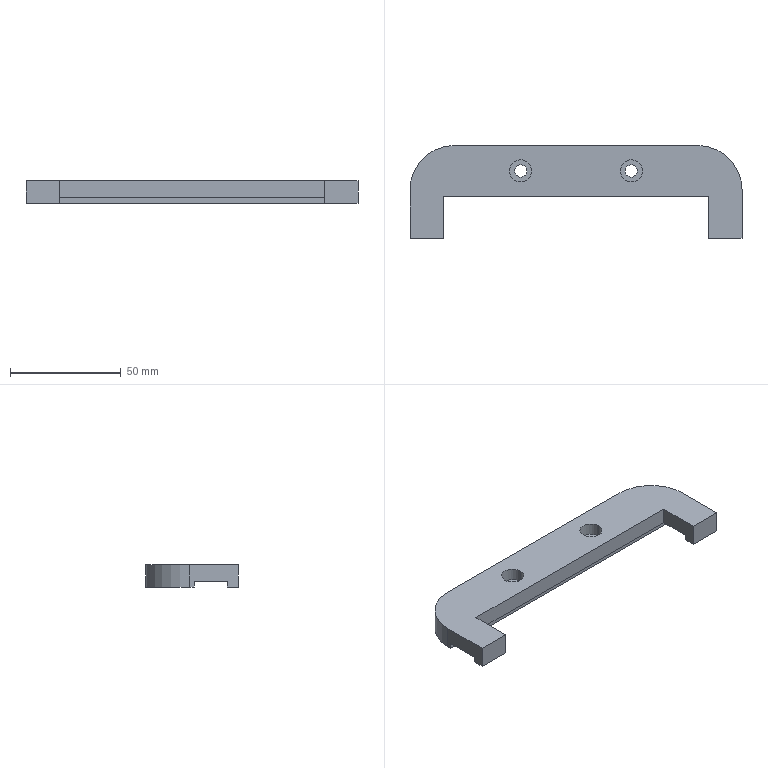Part | STEP file | X77-04403 | 1 solid | 28 faces | box 150 x 42 x 10 mm | volume 35959 mm3 | plane 18 | cylinder 10 | commonest cylinder face diameters 5.5 x4 10 x4 40 x2
STEP:
#1=CARTESIAN_POINT('',(45.,30.5,4.3));
#2=VERTEX_POINT('',#1);
#3=CARTESIAN_POINT('',(55.,30.5,4.3));
#4=VERTEX_POINT('',#3);
#5=CARTESIAN_POINT('',(50.,30.5,4.3));
#6=DIRECTION('',(0.,0.,1.));
#7=DIRECTION('',(1.,0.,0.));
#8=AXIS2_PLACEMENT_3D('',#5,#6,#7);
#9=CIRCLE('',#8,5.);
#10=EDGE_CURVE('',#2,#4,#9,.T.);
#11=ORIENTED_EDGE('',*,*,#10,.F.);
#12=CARTESIAN_POINT('',(45.,30.5,10.));
#13=VERTEX_POINT('',#12);
#14=CARTESIAN_POINT('',(45.,30.5,10.));
#15=DIRECTION('',(0.,0.,1.));
#16=VECTOR('',#15,1000.);
#17=LINE('',#14,#16);
#18=EDGE_CURVE('',#2,#13,#17,.T.);
#19=ORIENTED_EDGE('',*,*,#18,.T.);
#20=CARTESIAN_POINT('',(55.,30.5,10.));
#21=VERTEX_POINT('',#20);
#22=CARTESIAN_POINT('',(50.,30.5,10.));
#23=DIRECTION('',(0.,0.,1.));
#24=DIRECTION('',(1.,0.,0.));
#25=AXIS2_PLACEMENT_3D('',#22,#23,#24);
#26=CIRCLE('',#25,5.);
#27=EDGE_CURVE('',#13,#21,#26,.T.);
#28=ORIENTED_EDGE('',*,*,#27,.T.);
#29=CARTESIAN_POINT('',(55.,30.5,10.));
#30=DIRECTION('',(0.,0.,1.));
#31=VECTOR('',#30,1000.);
#32=LINE('',#29,#31);
#33=EDGE_CURVE('',#4,#21,#32,.T.);
#34=ORIENTED_EDGE('',*,*,#33,.F.);
#35=EDGE_LOOP('',(#11,#19,#28,#34));
#36=FACE_OUTER_BOUND('',#35,.T.);
#37=CARTESIAN_POINT('',(50.,30.5,10.));
#38=DIRECTION('',(0.,0.,1.));
#39=DIRECTION('',(1.,0.,0.));
#40=AXIS2_PLACEMENT_3D('',#37,#38,#39);
#41=CYLINDRICAL_SURFACE('',#40,5.);
#42=ADVANCED_FACE('',(#36),#41,.F.);
#43=CARTESIAN_POINT('',(47.25,30.5,0.));
#44=VERTEX_POINT('',#43);
#45=CARTESIAN_POINT('',(52.75,30.5,0.));
#46=VERTEX_POINT('',#45);
#47=CARTESIAN_POINT('',(50.,30.5,0.));
#48=DIRECTION('',(0.,0.,1.));
#49=DIRECTION('',(1.,0.,0.));
#50=AXIS2_PLACEMENT_3D('',#47,#48,#49);
#51=CIRCLE('',#50,2.75);
#52=EDGE_CURVE('',#44,#46,#51,.T.);
#53=ORIENTED_EDGE('',*,*,#52,.F.);
#54=CARTESIAN_POINT('',(47.25,30.5,4.3));
#55=VERTEX_POINT('',#54);
#56=CARTESIAN_POINT('',(47.25,30.5,10.));
#57=DIRECTION('',(0.,0.,1.));
#58=VECTOR('',#57,1000.);
#59=LINE('',#56,#58);
#60=EDGE_CURVE('',#44,#55,#59,.T.);
#61=ORIENTED_EDGE('',*,*,#60,.T.);
#62=CARTESIAN_POINT('',(52.75,30.5,4.3));
#63=VERTEX_POINT('',#62);
#64=CARTESIAN_POINT('',(50.,30.5,4.3));
#65=DIRECTION('',(0.,0.,1.));
#66=DIRECTION('',(1.,0.,0.));
#67=AXIS2_PLACEMENT_3D('',#64,#65,#66);
#68=CIRCLE('',#67,2.75);
#69=EDGE_CURVE('',#55,#63,#68,.T.);
#70=ORIENTED_EDGE('',*,*,#69,.T.);
#71=CARTESIAN_POINT('',(52.75,30.5,10.));
#72=DIRECTION('',(0.,0.,1.));
#73=VECTOR('',#72,1000.);
#74=LINE('',#71,#73);
#75=EDGE_CURVE('',#46,#63,#74,.T.);
#76=ORIENTED_EDGE('',*,*,#75,.F.);
#77=EDGE_LOOP('',(#53,#61,#70,#76));
#78=FACE_OUTER_BOUND('',#77,.T.);
#79=CARTESIAN_POINT('',(50.,30.5,10.));
#80=DIRECTION('',(0.,0.,1.));
#81=DIRECTION('',(1.,0.,0.));
#82=AXIS2_PLACEMENT_3D('',#79,#80,#81);
#83=CYLINDRICAL_SURFACE('',#82,2.75);
#84=ADVANCED_FACE('',(#78),#83,.F.);
#85=CARTESIAN_POINT('',(95.,30.5,4.3));
#86=VERTEX_POINT('',#85);
#87=CARTESIAN_POINT('',(105.,30.5,4.3));
#88=VERTEX_POINT('',#87);
#89=CARTESIAN_POINT('',(100.,30.5,4.3));
#90=DIRECTION('',(0.,0.,1.));
#91=DIRECTION('',(1.,0.,0.));
#92=AXIS2_PLACEMENT_3D('',#89,#90,#91);
#93=CIRCLE('',#92,5.);
#94=EDGE_CURVE('',#86,#88,#93,.T.);
#95=ORIENTED_EDGE('',*,*,#94,.F.);
#96=CARTESIAN_POINT('',(95.,30.5,10.));
#97=VERTEX_POINT('',#96);
#98=CARTESIAN_POINT('',(95.,30.5,10.));
#99=DIRECTION('',(0.,0.,1.));
#100=VECTOR('',#99,1000.);
#101=LINE('',#98,#100);
#102=EDGE_CURVE('',#86,#97,#101,.T.);
#103=ORIENTED_EDGE('',*,*,#102,.T.);
#104=CARTESIAN_POINT('',(105.,30.5,10.));
#105=VERTEX_POINT('',#104);
#106=CARTESIAN_POINT('',(100.,30.5,10.));
#107=DIRECTION('',(0.,0.,1.));
#108=DIRECTION('',(1.,0.,0.));
#109=AXIS2_PLACEMENT_3D('',#106,#107,#108);
#110=CIRCLE('',#109,5.);
#111=EDGE_CURVE('',#97,#105,#110,.T.);
#112=ORIENTED_EDGE('',*,*,#111,.T.);
#113=CARTESIAN_POINT('',(105.,30.5,10.));
#114=DIRECTION('',(0.,0.,1.));
#115=VECTOR('',#114,1000.);
#116=LINE('',#113,#115);
#117=EDGE_CURVE('',#88,#105,#116,.T.);
#118=ORIENTED_EDGE('',*,*,#117,.F.);
#119=EDGE_LOOP('',(#95,#103,#112,#118));
#120=FACE_OUTER_BOUND('',#119,.T.);
#121=CARTESIAN_POINT('',(100.,30.5,10.));
#122=DIRECTION('',(0.,0.,1.));
#123=DIRECTION('',(1.,0.,0.));
#124=AXIS2_PLACEMENT_3D('',#121,#122,#123);
#125=CYLINDRICAL_SURFACE('',#124,5.);
#126=ADVANCED_FACE('',(#120),#125,.F.);
#127=CARTESIAN_POINT('',(97.25,30.5,0.));
#128=VERTEX_POINT('',#127);
#129=CARTESIAN_POINT('',(102.75,30.5,0.));
#130=VERTEX_POINT('',#129);
#131=CARTESIAN_POINT('',(100.,30.5,0.));
#132=DIRECTION('',(0.,0.,1.));
#133=DIRECTION('',(1.,0.,0.));
#134=AXIS2_PLACEMENT_3D('',#131,#132,#133);
#135=CIRCLE('',#134,2.75);
#136=EDGE_CURVE('',#128,#130,#135,.T.);
#137=ORIENTED_EDGE('',*,*,#136,.F.);
#138=CARTESIAN_POINT('',(97.25,30.5,4.3));
#139=VERTEX_POINT('',#138);
#140=CARTESIAN_POINT('',(97.25,30.5,10.));
#141=DIRECTION('',(0.,0.,1.));
#142=VECTOR('',#141,1000.);
#143=LINE('',#140,#142);
#144=EDGE_CURVE('',#128,#139,#143,.T.);
#145=ORIENTED_EDGE('',*,*,#144,.T.);
#146=CARTESIAN_POINT('',(102.75,30.5,4.3));
#147=VERTEX_POINT('',#146);
#148=CARTESIAN_POINT('',(100.,30.5,4.3));
#149=DIRECTION('',(0.,0.,1.));
#150=DIRECTION('',(1.,0.,0.));
#151=AXIS2_PLACEMENT_3D('',#148,#149,#150);
#152=CIRCLE('',#151,2.75);
#153=EDGE_CURVE('',#139,#147,#152,.T.);
#154=ORIENTED_EDGE('',*,*,#153,.T.);
#155=CARTESIAN_POINT('',(102.75,30.5,10.));
#156=DIRECTION('',(0.,0.,1.));
#157=VECTOR('',#156,1000.);
#158=LINE('',#155,#157);
#159=EDGE_CURVE('',#130,#147,#158,.T.);
#160=ORIENTED_EDGE('',*,*,#159,.F.);
#161=EDGE_LOOP('',(#137,#145,#154,#160));
#162=FACE_OUTER_BOUND('',#161,.T.);
#163=CARTESIAN_POINT('',(100.,30.5,10.));
#164=DIRECTION('',(0.,0.,1.));
#165=DIRECTION('',(1.,0.,0.));
#166=AXIS2_PLACEMENT_3D('',#163,#164,#165);
#167=CYLINDRICAL_SURFACE('',#166,2.75);
#168=ADVANCED_FACE('',(#162),#167,.F.);
#169=CARTESIAN_POINT('',(150.,5.,0.));
#170=VERTEX_POINT('',#169);
#171=CARTESIAN_POINT('',(135.,5.,0.));
#172=VERTEX_POINT('',#171);
#173=CARTESIAN_POINT('',(0.,5.,0.));
#174=DIRECTION('',(-1.,0.,0.));
#175=VECTOR('',#174,1000.);
#176=LINE('',#173,#175);
#177=EDGE_CURVE('',#170,#172,#176,.T.);
#178=ORIENTED_EDGE('',*,*,#177,.F.);
#179=CARTESIAN_POINT('',(150.,0.,0.));
#180=VERTEX_POINT('',#179);
#181=CARTESIAN_POINT('',(150.,0.,0.));
#182=DIRECTION('',(0.,1.,0.));
#183=VECTOR('',#182,1000.);
#184=LINE('',#181,#183);
#185=EDGE_CURVE('',#180,#170,#184,.T.);
#186=ORIENTED_EDGE('',*,*,#185,.F.);
#187=CARTESIAN_POINT('',(135.,0.,0.));
#188=VERTEX_POINT('',#187);
#189=CARTESIAN_POINT('',(135.,0.,0.));
#190=DIRECTION('',(1.,0.,0.));
#191=VECTOR('',#190,1000.);
#192=LINE('',#189,#191);
#193=EDGE_CURVE('',#188,#180,#192,.T.);
#194=ORIENTED_EDGE('',*,*,#193,.F.);
#195=CARTESIAN_POINT('',(135.,0.,0.));
#196=DIRECTION('',(0.,-1.,0.));
#197=VECTOR('',#196,1000.);
#198=LINE('',#195,#197);
#199=EDGE_CURVE('',#172,#188,#198,.T.);
#200=ORIENTED_EDGE('',*,*,#199,.F.);
#201=EDGE_LOOP('',(#178,#186,#194,#200));
#202=FACE_OUTER_BOUND('',#201,.T.);
#203=CARTESIAN_POINT('',(0.,42.,0.));
#204=DIRECTION('',(0.,0.,-1.));
#205=DIRECTION('',(-1.,0.,0.));
#206=AXIS2_PLACEMENT_3D('',#203,#204,#205);
#207=PLANE('',#206);
#208=ADVANCED_FACE('',(#202),#207,.T.);
#209=CARTESIAN_POINT('',(15.,5.,0.));
#210=VERTEX_POINT('',#209);
#211=CARTESIAN_POINT('',(0.,5.,0.));
#212=VERTEX_POINT('',#211);
#213=CARTESIAN_POINT('',(0.,5.,0.));
#214=DIRECTION('',(-1.,0.,0.));
#215=VECTOR('',#214,1000.);
#216=LINE('',#213,#215);
#217=EDGE_CURVE('',#210,#212,#216,.T.);
#218=ORIENTED_EDGE('',*,*,#217,.F.);
#219=CARTESIAN_POINT('',(15.,0.,0.));
#220=VERTEX_POINT('',#219);
#221=CARTESIAN_POINT('',(15.,0.,0.));
#222=DIRECTION('',(0.,1.,0.));
#223=VECTOR('',#222,1000.);
#224=LINE('',#221,#223);
#225=EDGE_CURVE('',#220,#210,#224,.T.);
#226=ORIENTED_EDGE('',*,*,#225,.F.);
#227=CARTESIAN_POINT('',(0.,0.,0.));
#228=VERTEX_POINT('',#227);
#229=CARTESIAN_POINT('',(0.,0.,0.));
#230=DIRECTION('',(1.,0.,0.));
#231=VECTOR('',#230,1000.);
#232=LINE('',#229,#231);
#233=EDGE_CURVE('',#228,#220,#232,.T.);
#234=ORIENTED_EDGE('',*,*,#233,.F.);
#235=CARTESIAN_POINT('',(0.,0.,0.));
#236=DIRECTION('',(0.,-1.,0.));
#237=VECTOR('',#236,1000.);
#238=LINE('',#235,#237);
#239=EDGE_CURVE('',#212,#228,#238,.T.);
#240=ORIENTED_EDGE('',*,*,#239,.F.);
#241=EDGE_LOOP('',(#218,#226,#234,#240));
#242=FACE_OUTER_BOUND('',#241,.T.);
#243=CARTESIAN_POINT('',(0.,42.,0.));
#244=DIRECTION('',(0.,0.,-1.));
#245=DIRECTION('',(-1.,0.,0.));
#246=AXIS2_PLACEMENT_3D('',#243,#244,#245);
#247=PLANE('',#246);
#248=ADVANCED_FACE('',(#242),#247,.T.);
#249=CARTESIAN_POINT('',(0.,22.,10.));
#250=VERTEX_POINT('',#249);
#251=CARTESIAN_POINT('',(0.,0.,10.));
#252=VERTEX_POINT('',#251);
#253=CARTESIAN_POINT('',(0.,0.,10.));
#254=DIRECTION('',(0.,-1.,0.));
#255=VECTOR('',#254,1000.);
#256=LINE('',#253,#255);
#257=EDGE_CURVE('',#250,#252,#256,.T.);
#258=ORIENTED_EDGE('',*,*,#257,.F.);
#259=CARTESIAN_POINT('',(0.,22.,0.));
#260=VERTEX_POINT('',#259);
#261=CARTESIAN_POINT('',(0.,22.,10.));
#262=DIRECTION('',(0.,0.,-1.));
#263=VECTOR('',#262,1000.);
#264=LINE('',#261,#263);
#265=EDGE_CURVE('',#250,#260,#264,.T.);
#266=ORIENTED_EDGE('',*,*,#265,.T.);
#267=CARTESIAN_POINT('',(0.,20.,0.));
#268=VERTEX_POINT('',#267);
#269=CARTESIAN_POINT('',(0.,0.,0.));
#270=DIRECTION('',(0.,-1.,0.));
#271=VECTOR('',#270,1000.);
#272=LINE('',#269,#271);
#273=EDGE_CURVE('',#260,#268,#272,.T.);
#274=ORIENTED_EDGE('',*,*,#273,.T.);
#275=CARTESIAN_POINT('',(0.,20.,2.5));
#276=VERTEX_POINT('',#275);
#277=CARTESIAN_POINT('',(0.,20.,10.));
#278=DIRECTION('',(0.,0.,1.));
#279=VECTOR('',#278,1000.);
#280=LINE('',#277,#279);
#281=EDGE_CURVE('',#268,#276,#280,.T.);
#282=ORIENTED_EDGE('',*,*,#281,.T.);
#283=CARTESIAN_POINT('',(0.,5.,2.5));
#284=VERTEX_POINT('',#283);
#285=CARTESIAN_POINT('',(0.,0.,2.5));
#286=DIRECTION('',(0.,-1.,0.));
#287=VECTOR('',#286,1000.);
#288=LINE('',#285,#287);
#289=EDGE_CURVE('',#276,#284,#288,.T.);
#290=ORIENTED_EDGE('',*,*,#289,.T.);
#291=CARTESIAN_POINT('',(0.,5.,10.));
#292=DIRECTION('',(0.,0.,-1.));
#293=VECTOR('',#292,1000.);
#294=LINE('',#291,#293);
#295=EDGE_CURVE('',#284,#212,#294,.T.);
#296=ORIENTED_EDGE('',*,*,#295,.T.);
#297=ORIENTED_EDGE('',*,*,#239,.T.);
#298=CARTESIAN_POINT('',(0.,0.,10.));
#299=DIRECTION('',(0.,0.,-1.));
#300=VECTOR('',#299,1000.);
#301=LINE('',#298,#300);
#302=EDGE_CURVE('',#252,#228,#301,.T.);
#303=ORIENTED_EDGE('',*,*,#302,.F.);
#304=EDGE_LOOP('',(#258,#266,#274,#282,#290,#296,#297,#303));
#305=FACE_OUTER_BOUND('',#304,.T.);
#306=CARTESIAN_POINT('',(0.,0.,10.));
#307=DIRECTION('',(1.,0.,0.));
#308=DIRECTION('',(0.,0.,-1.));
#309=AXIS2_PLACEMENT_3D('',#306,#307,#308);
#310=PLANE('',#309);
#311=ADVANCED_FACE('',(#305),#310,.F.);
#312=ORIENTED_EDGE('',*,*,#233,.T.);
#313=CARTESIAN_POINT('',(15.,0.,10.));
#314=VERTEX_POINT('',#313);
#315=CARTESIAN_POINT('',(15.,0.,10.));
#316=DIRECTION('',(0.,0.,-1.));
#317=VECTOR('',#316,1000.);
#318=LINE('',#315,#317);
#319=EDGE_CURVE('',#314,#220,#318,.T.);
#320=ORIENTED_EDGE('',*,*,#319,.F.);
#321=CARTESIAN_POINT('',(0.,0.,10.));
#322=DIRECTION('',(1.,0.,0.));
#323=VECTOR('',#322,1000.);
#324=LINE('',#321,#323);
#325=EDGE_CURVE('',#252,#314,#324,.T.);
#326=ORIENTED_EDGE('',*,*,#325,.F.);
#327=ORIENTED_EDGE('',*,*,#302,.T.);
#328=EDGE_LOOP('',(#312,#320,#326,#327));
#329=FACE_OUTER_BOUND('',#328,.T.);
#330=CARTESIAN_POINT('',(0.,0.,10.));
#331=DIRECTION('',(0.,1.,0.));
#332=DIRECTION('',(0.,0.,1.));
#333=AXIS2_PLACEMENT_3D('',#330,#331,#332);
#334=PLANE('',#333);
#335=ADVANCED_FACE('',(#329),#334,.F.);
#336=ORIENTED_EDGE('',*,*,#225,.T.);
#337=CARTESIAN_POINT('',(15.,5.,2.5));
#338=VERTEX_POINT('',#337);
#339=CARTESIAN_POINT('',(15.,5.,10.));
#340=DIRECTION('',(0.,0.,1.));
#341=VECTOR('',#340,1000.);
#342=LINE('',#339,#341);
#343=EDGE_CURVE('',#210,#338,#342,.T.);
#344=ORIENTED_EDGE('',*,*,#343,.T.);
#345=CARTESIAN_POINT('',(15.,19.,2.5));
#346=VERTEX_POINT('',#345);
#347=CARTESIAN_POINT('',(15.,0.,2.5));
#348=DIRECTION('',(0.,1.,0.));
#349=VECTOR('',#348,1000.);
#350=LINE('',#347,#349);
#351=EDGE_CURVE('',#338,#346,#350,.T.);
#352=ORIENTED_EDGE('',*,*,#351,.T.);
#353=CARTESIAN_POINT('',(15.,19.,10.));
#354=VERTEX_POINT('',#353);
#355=CARTESIAN_POINT('',(15.,19.,10.));
#356=DIRECTION('',(0.,0.,-1.));
#357=VECTOR('',#356,1000.);
#358=LINE('',#355,#357);
#359=EDGE_CURVE('',#354,#346,#358,.T.);
#360=ORIENTED_EDGE('',*,*,#359,.F.);
#361=CARTESIAN_POINT('',(15.,0.,10.));
#362=DIRECTION('',(0.,1.,0.));
#363=VECTOR('',#362,1000.);
#364=LINE('',#361,#363);
#365=EDGE_CURVE('',#314,#354,#364,.T.);
#366=ORIENTED_EDGE('',*,*,#365,.F.);
#367=ORIENTED_EDGE('',*,*,#319,.T.);
#368=EDGE_LOOP('',(#336,#344,#352,#360,#366,#367));
#369=FACE_OUTER_BOUND('',#368,.T.);
#370=CARTESIAN_POINT('',(15.,0.,10.));
#371=DIRECTION('',(-1.,0.,0.));
#372=DIRECTION('',(0.,0.,1.));
#373=AXIS2_PLACEMENT_3D('',#370,#371,#372);
#374=PLANE('',#373);
#375=ADVANCED_FACE('',(#369),#374,.F.);
#376=ORIENTED_EDGE('',*,*,#359,.T.);
#377=CARTESIAN_POINT('',(135.,19.,2.5));
#378=VERTEX_POINT('',#377);
#379=CARTESIAN_POINT('',(15.,19.,2.5));
#380=DIRECTION('',(1.,0.,0.));
#381=VECTOR('',#380,1000.);
#382=LINE('',#379,#381);
#383=EDGE_CURVE('',#346,#378,#382,.T.);
#384=ORIENTED_EDGE('',*,*,#383,.T.);
#385=CARTESIAN_POINT('',(135.,19.,10.));
#386=VERTEX_POINT('',#385);
#387=CARTESIAN_POINT('',(135.,19.,10.));
#388=DIRECTION('',(0.,0.,-1.));
#389=VECTOR('',#388,1000.);
#390=LINE('',#387,#389);
#391=EDGE_CURVE('',#386,#378,#390,.T.);
#392=ORIENTED_EDGE('',*,*,#391,.F.);
#393=CARTESIAN_POINT('',(15.,19.,10.));
#394=DIRECTION('',(1.,0.,0.));
#395=VECTOR('',#394,1000.);
#396=LINE('',#393,#395);
#397=EDGE_CURVE('',#354,#386,#396,.T.);
#398=ORIENTED_EDGE('',*,*,#397,.F.);
#399=EDGE_LOOP('',(#376,#384,#392,#398));
#400=FACE_OUTER_BOUND('',#399,.T.);
#401=CARTESIAN_POINT('',(15.,19.,10.));
#402=DIRECTION('',(0.,1.,0.));
#403=DIRECTION('',(-1.,0.,0.));
#404=AXIS2_PLACEMENT_3D('',#401,#402,#403);
#405=PLANE('',#404);
#406=ADVANCED_FACE('',(#400),#405,.F.);
#407=CARTESIAN_POINT('',(135.,5.,2.5));
#408=VERTEX_POINT('',#407);
#409=CARTESIAN_POINT('',(135.,0.,2.5));
#410=DIRECTION('',(0.,-1.,0.));
#411=VECTOR('',#410,1000.);
#412=LINE('',#409,#411);
#413=EDGE_CURVE('',#378,#408,#412,.T.);
#414=ORIENTED_EDGE('',*,*,#413,.T.);
#415=CARTESIAN_POINT('',(135.,5.,10.));
#416=DIRECTION('',(0.,0.,-1.));
#417=VECTOR('',#416,1000.);
#418=LINE('',#415,#417);
#419=EDGE_CURVE('',#408,#172,#418,.T.);
#420=ORIENTED_EDGE('',*,*,#419,.T.);
#421=ORIENTED_EDGE('',*,*,#199,.T.);
#422=CARTESIAN_POINT('',(135.,0.,10.));
#423=VERTEX_POINT('',#422);
#424=CARTESIAN_POINT('',(135.,0.,10.));
#425=DIRECTION('',(0.,0.,-1.));
#426=VECTOR('',#425,1000.);
#427=LINE('',#424,#426);
#428=EDGE_CURVE('',#423,#188,#427,.T.);
#429=ORIENTED_EDGE('',*,*,#428,.F.);
#430=CARTESIAN_POINT('',(135.,0.,10.));
#431=DIRECTION('',(0.,-1.,0.));
#432=VECTOR('',#431,1000.);
#433=LINE('',#430,#432);
#434=EDGE_CURVE('',#386,#423,#433,.T.);
#435=ORIENTED_EDGE('',*,*,#434,.F.);
#436=ORIENTED_EDGE('',*,*,#391,.T.);
#437=EDGE_LOOP('',(#414,#420,#421,#429,#435,#436));
#438=FACE_OUTER_BOUND('',#437,.T.);
#439=CARTESIAN_POINT('',(135.,0.,10.));
#440=DIRECTION('',(1.,0.,0.));
#441=DIRECTION('',(0.,0.,-1.));
#442=AXIS2_PLACEMENT_3D('',#439,#440,#441);
#443=PLANE('',#442);
#444=ADVANCED_FACE('',(#438),#443,.F.);
#445=ORIENTED_EDGE('',*,*,#193,.T.);
#446=CARTESIAN_POINT('',(150.,0.,10.));
#447=VERTEX_POINT('',#446);
#448=CARTESIAN_POINT('',(150.,0.,10.));
#449=DIRECTION('',(0.,0.,-1.));
#450=VECTOR('',#449,1000.);
#451=LINE('',#448,#450);
#452=EDGE_CURVE('',#447,#180,#451,.T.);
#453=ORIENTED_EDGE('',*,*,#452,.F.);
#454=CARTESIAN_POINT('',(135.,0.,10.));
#455=DIRECTION('',(1.,0.,0.));
#456=VECTOR('',#455,1000.);
#457=LINE('',#454,#456);
#458=EDGE_CURVE('',#423,#447,#457,.T.);
#459=ORIENTED_EDGE('',*,*,#458,.F.);
#460=ORIENTED_EDGE('',*,*,#428,.T.);
#461=EDGE_LOOP('',(#445,#453,#459,#460));
#462=FACE_OUTER_BOUND('',#461,.T.);
#463=CARTESIAN_POINT('',(135.,0.,10.));
#464=DIRECTION('',(0.,1.,0.));
#465=DIRECTION('',(0.,0.,1.));
#466=AXIS2_PLACEMENT_3D('',#463,#464,#465);
#467=PLANE('',#466);
#468=ADVANCED_FACE('',(#462),#467,.F.);
#469=CARTESIAN_POINT('',(150.,20.,0.));
#470=VERTEX_POINT('',#469);
#471=CARTESIAN_POINT('',(150.,22.,0.));
#472=VERTEX_POINT('',#471);
#473=CARTESIAN_POINT('',(150.,0.,0.));
#474=DIRECTION('',(0.,1.,0.));
#475=VECTOR('',#474,1000.);
#476=LINE('',#473,#475);
#477=EDGE_CURVE('',#470,#472,#476,.T.);
#478=ORIENTED_EDGE('',*,*,#477,.T.);
#479=CARTESIAN_POINT('',(150.,22.,10.));
#480=VERTEX_POINT('',#479);
#481=CARTESIAN_POINT('',(150.,22.,10.));
#482=DIRECTION('',(0.,0.,1.));
#483=VECTOR('',#482,1000.);
#484=LINE('',#481,#483);
#485=EDGE_CURVE('',#472,#480,#484,.T.);
#486=ORIENTED_EDGE('',*,*,#485,.T.);
#487=CARTESIAN_POINT('',(150.,0.,10.));
#488=DIRECTION('',(0.,1.,0.));
#489=VECTOR('',#488,1000.);
#490=LINE('',#487,#489);
#491=EDGE_CURVE('',#447,#480,#490,.T.);
#492=ORIENTED_EDGE('',*,*,#491,.F.);
#493=ORIENTED_EDGE('',*,*,#452,.T.);
#494=ORIENTED_EDGE('',*,*,#185,.T.);
#495=CARTESIAN_POINT('',(150.,5.,2.5));
#496=VERTEX_POINT('',#495);
#497=CARTESIAN_POINT('',(150.,5.,0.));
#498=DIRECTION('',(0.,0.,-1.));
#499=VECTOR('',#498,1000.);
#500=LINE('',#497,#499);
#501=EDGE_CURVE('',#496,#170,#500,.T.);
#502=ORIENTED_EDGE('',*,*,#501,.F.);
#503=CARTESIAN_POINT('',(150.,20.,2.5));
#504=VERTEX_POINT('',#503);
#505=CARTESIAN_POINT('',(150.,5.,2.5));
#506=DIRECTION('',(0.,-1.,0.));
#507=VECTOR('',#506,1000.);
#508=LINE('',#505,#507);
#509=EDGE_CURVE('',#504,#496,#508,.T.);
#510=ORIENTED_EDGE('',*,*,#509,.F.);
#511=CARTESIAN_POINT('',(150.,20.,0.));
#512=DIRECTION('',(0.,0.,1.));
#513=VECTOR('',#512,1000.);
#514=LINE('',#511,#513);
#515=EDGE_CURVE('',#470,#504,#514,.T.);
#516=ORIENTED_EDGE('',*,*,#515,.F.);
#517=EDGE_LOOP('',(#478,#486,#492,#493,#494,#502,#510,#516));
#518=FACE_OUTER_BOUND('',#517,.T.);
#519=CARTESIAN_POINT('',(150.,0.,10.));
#520=DIRECTION('',(-1.,0.,0.));
#521=DIRECTION('',(0.,0.,1.));
#522=AXIS2_PLACEMENT_3D('',#519,#520,#521);
#523=PLANE('',#522);
#524=ADVANCED_FACE('',(#518),#523,.F.);
#525=CARTESIAN_POINT('',(130.,42.,0.));
#526=VERTEX_POINT('',#525);
#527=CARTESIAN_POINT('',(20.,42.,0.));
#528=VERTEX_POINT('',#527);
#529=CARTESIAN_POINT('',(0.,42.,0.));
#530=DIRECTION('',(-1.,0.,0.));
#531=VECTOR('',#530,1000.);
#532=LINE('',#529,#531);
#533=EDGE_CURVE('',#526,#528,#532,.T.);
#534=ORIENTED_EDGE('',*,*,#533,.T.);
#535=CARTESIAN_POINT('',(20.,42.,10.));
#536=VERTEX_POINT('',#535);
#537=CARTESIAN_POINT('',(20.,42.,10.));
#538=DIRECTION('',(0.,0.,1.));
#539=VECTOR('',#538,1000.);
#540=LINE('',#537,#539);
#541=EDGE_CURVE('',#528,#536,#540,.T.);
#542=ORIENTED_EDGE('',*,*,#541,.T.);
#543=CARTESIAN_POINT('',(130.,42.,10.));
#544=VERTEX_POINT('',#543);
#545=CARTESIAN_POINT('',(0.,42.,10.));
#546=DIRECTION('',(-1.,0.,0.));
#547=VECTOR('',#546,1000.);
#548=LINE('',#545,#547);
#549=EDGE_CURVE('',#544,#536,#548,.T.);
#550=ORIENTED_EDGE('',*,*,#549,.F.);
#551=CARTESIAN_POINT('',(130.,42.,10.));
#552=DIRECTION('',(0.,0.,-1.));
#553=VECTOR('',#552,1000.);
#554=LINE('',#551,#553);
#555=EDGE_CURVE('',#544,#526,#554,.T.);
#556=ORIENTED_EDGE('',*,*,#555,.T.);
#557=EDGE_LOOP('',(#534,#542,#550,#556));
#558=FACE_OUTER_BOUND('',#557,.T.);
#559=CARTESIAN_POINT('',(0.,42.,10.));
#560=DIRECTION('',(0.,-1.,0.));
#561=DIRECTION('',(1.,0.,0.));
#562=AXIS2_PLACEMENT_3D('',#559,#560,#561);
#563=PLANE('',#562);
#564=ADVANCED_FACE('',(#558),#563,.F.);
#565=CARTESIAN_POINT('',(50.,30.5,10.));
#566=DIRECTION('',(0.,0.,1.));
#567=DIRECTION('',(1.,0.,0.));
#568=AXIS2_PLACEMENT_3D('',#565,#566,#567);
#569=CIRCLE('',#568,5.);
#570=EDGE_CURVE('',#21,#13,#569,.T.);
#571=ORIENTED_EDGE('',*,*,#570,.F.);
#572=ORIENTED_EDGE('',*,*,#27,.F.);
#573=EDGE_LOOP('',(#571,#572));
#574=FACE_BOUND('',#573,.T.);
#575=CARTESIAN_POINT('',(100.,30.5,10.));
#576=DIRECTION('',(0.,0.,1.));
#577=DIRECTION('',(1.,0.,0.));
#578=AXIS2_PLACEMENT_3D('',#575,#576,#577);
#579=CIRCLE('',#578,5.);
#580=EDGE_CURVE('',#105,#97,#579,.T.);
#581=ORIENTED_EDGE('',*,*,#580,.F.);
#582=ORIENTED_EDGE('',*,*,#111,.F.);
#583=EDGE_LOOP('',(#581,#582));
#584=FACE_BOUND('',#583,.T.);
#585=ORIENTED_EDGE('',*,*,#549,.T.);
#586=CARTESIAN_POINT('',(20.,22.,10.));
#587=DIRECTION('',(0.,0.,1.));
#588=DIRECTION('',(-1.,0.,0.));
#589=AXIS2_PLACEMENT_3D('',#586,#587,#588);
#590=CIRCLE('',#589,20.);
#591=EDGE_CURVE('',#536,#250,#590,.T.);
#592=ORIENTED_EDGE('',*,*,#591,.T.);
#593=ORIENTED_EDGE('',*,*,#257,.T.);
#594=ORIENTED_EDGE('',*,*,#325,.T.);
#595=ORIENTED_EDGE('',*,*,#365,.T.);
#596=ORIENTED_EDGE('',*,*,#397,.T.);
#597=ORIENTED_EDGE('',*,*,#434,.T.);
#598=ORIENTED_EDGE('',*,*,#458,.T.);
#599=ORIENTED_EDGE('',*,*,#491,.T.);
#600=CARTESIAN_POINT('',(130.,22.,10.));
#601=DIRECTION('',(0.,0.,1.));
#602=DIRECTION('',(-1.,0.,0.));
#603=AXIS2_PLACEMENT_3D('',#600,#601,#602);
#604=CIRCLE('',#603,20.);
#605=EDGE_CURVE('',#480,#544,#604,.T.);
#606=ORIENTED_EDGE('',*,*,#605,.T.);
#607=EDGE_LOOP('',(#585,#592,#593,#594,#595,#596,#597,#598,#599,#606));
#608=FACE_OUTER_BOUND('',#607,.T.);
#609=CARTESIAN_POINT('',(0.,42.,10.));
#610=DIRECTION('',(0.,0.,-1.));
#611=DIRECTION('',(-1.,0.,0.));
#612=AXIS2_PLACEMENT_3D('',#609,#610,#611);
#613=PLANE('',#612);
#614=ADVANCED_FACE('',(#574,#584,#608),#613,.F.);
#615=CARTESIAN_POINT('',(50.,30.5,0.));
#616=DIRECTION('',(0.,0.,1.));
#617=DIRECTION('',(1.,0.,0.));
#618=AXIS2_PLACEMENT_3D('',#615,#616,#617);
#619=CIRCLE('',#618,2.75);
#620=EDGE_CURVE('',#46,#44,#619,.T.);
#621=ORIENTED_EDGE('',*,*,#620,.T.);
#622=ORIENTED_EDGE('',*,*,#52,.T.);
#623=EDGE_LOOP('',(#621,#622));
#624=FACE_BOUND('',#623,.T.);
#625=CARTESIAN_POINT('',(100.,30.5,0.));
#626=DIRECTION('',(0.,0.,1.));
#627=DIRECTION('',(1.,0.,0.));
#628=AXIS2_PLACEMENT_3D('',#625,#626,#627);
#629=CIRCLE('',#628,2.75);
#630=EDGE_CURVE('',#130,#128,#629,.T.);
#631=ORIENTED_EDGE('',*,*,#630,.T.);
#632=ORIENTED_EDGE('',*,*,#136,.T.);
#633=EDGE_LOOP('',(#631,#632));
#634=FACE_BOUND('',#633,.T.);
#635=ORIENTED_EDGE('',*,*,#273,.F.);
#636=CARTESIAN_POINT('',(20.,22.,0.));
#637=DIRECTION('',(0.,0.,-1.));
#638=DIRECTION('',(-1.,0.,0.));
#639=AXIS2_PLACEMENT_3D('',#636,#637,#638);
#640=CIRCLE('',#639,20.);
#641=EDGE_CURVE('',#260,#528,#640,.T.);
#642=ORIENTED_EDGE('',*,*,#641,.T.);
#643=ORIENTED_EDGE('',*,*,#533,.F.);
#644=CARTESIAN_POINT('',(130.,22.,0.));
#645=DIRECTION('',(0.,0.,-1.));
#646=DIRECTION('',(-1.,0.,0.));
#647=AXIS2_PLACEMENT_3D('',#644,#645,#646);
#648=CIRCLE('',#647,20.);
#649=EDGE_CURVE('',#526,#472,#648,.T.);
#650=ORIENTED_EDGE('',*,*,#649,.T.);
#651=ORIENTED_EDGE('',*,*,#477,.F.);
#652=CARTESIAN_POINT('',(0.,20.,0.));
#653=DIRECTION('',(1.,0.,0.));
#654=VECTOR('',#653,1000.);
#655=LINE('',#652,#654);
#656=EDGE_CURVE('',#268,#470,#655,.T.);
#657=ORIENTED_EDGE('',*,*,#656,.F.);
#658=EDGE_LOOP('',(#635,#642,#643,#650,#651,#657));
#659=FACE_OUTER_BOUND('',#658,.T.);
#660=CARTESIAN_POINT('',(0.,42.,0.));
#661=DIRECTION('',(0.,0.,-1.));
#662=DIRECTION('',(-1.,0.,0.));
#663=AXIS2_PLACEMENT_3D('',#660,#661,#662);
#664=PLANE('',#663);
#665=ADVANCED_FACE('',(#624,#634,#659),#664,.T.);
#666=CARTESIAN_POINT('',(-6.,20.,2.5));
#667=DIRECTION('',(1.,0.,0.));
#668=VECTOR('',#667,1000.);
#669=LINE('',#666,#668);
#670=EDGE_CURVE('',#276,#504,#669,.T.);
#671=ORIENTED_EDGE('',*,*,#670,.T.);
#672=ORIENTED_EDGE('',*,*,#509,.T.);
#673=CARTESIAN_POINT('',(-6.,5.,2.5));
#674=DIRECTION('',(1.,0.,0.));
#675=VECTOR('',#674,1000.);
#676=LINE('',#673,#675);
#677=EDGE_CURVE('',#408,#496,#676,.T.);
#678=ORIENTED_EDGE('',*,*,#677,.F.);
#679=ORIENTED_EDGE('',*,*,#413,.F.);
#680=ORIENTED_EDGE('',*,*,#383,.F.);
#681=ORIENTED_EDGE('',*,*,#351,.F.);
#682=CARTESIAN_POINT('',(-6.,5.,2.5));
#683=DIRECTION('',(1.,0.,0.));
#684=VECTOR('',#683,1000.);
#685=LINE('',#682,#684);
#686=EDGE_CURVE('',#284,#338,#685,.T.);
#687=ORIENTED_EDGE('',*,*,#686,.F.);
#688=ORIENTED_EDGE('',*,*,#289,.F.);
#689=EDGE_LOOP('',(#671,#672,#678,#679,#680,#681,#687,#688));
#690=FACE_OUTER_BOUND('',#689,.T.);
#691=CARTESIAN_POINT('',(-6.,5.,2.5));
#692=DIRECTION('',(0.,0.,1.));
#693=DIRECTION('',(1.,0.,0.));
#694=AXIS2_PLACEMENT_3D('',#691,#692,#693);
#695=PLANE('',#694);
#696=ADVANCED_FACE('',(#690),#695,.F.);
#697=ORIENTED_EDGE('',*,*,#686,.T.);
#698=ORIENTED_EDGE('',*,*,#343,.F.);
#699=ORIENTED_EDGE('',*,*,#217,.T.);
#700=ORIENTED_EDGE('',*,*,#295,.F.);
#701=EDGE_LOOP('',(#697,#698,#699,#700));
#702=FACE_OUTER_BOUND('',#701,.T.);
#703=CARTESIAN_POINT('',(-6.,5.,0.));
#704=DIRECTION('',(0.,-1.,0.));
#705=DIRECTION('',(0.,0.,-1.));
#706=AXIS2_PLACEMENT_3D('',#703,#704,#705);
#707=PLANE('',#706);
#708=ADVANCED_FACE('',(#702),#707,.F.);
#709=ORIENTED_EDGE('',*,*,#677,.T.);
#710=ORIENTED_EDGE('',*,*,#501,.T.);
#711=ORIENTED_EDGE('',*,*,#177,.T.);
#712=ORIENTED_EDGE('',*,*,#419,.F.);
#713=EDGE_LOOP('',(#709,#710,#711,#712));
#714=FACE_OUTER_BOUND('',#713,.T.);
#715=CARTESIAN_POINT('',(-6.,5.,0.));
#716=DIRECTION('',(0.,-1.,0.));
#717=DIRECTION('',(0.,0.,-1.));
#718=AXIS2_PLACEMENT_3D('',#715,#716,#717);
#719=PLANE('',#718);
#720=ADVANCED_FACE('',(#714),#719,.F.);
#721=ORIENTED_EDGE('',*,*,#656,.T.);
#722=ORIENTED_EDGE('',*,*,#515,.T.);
#723=ORIENTED_EDGE('',*,*,#670,.F.);
#724=ORIENTED_EDGE('',*,*,#281,.F.);
#725=EDGE_LOOP('',(#721,#722,#723,#724));
#726=FACE_OUTER_BOUND('',#725,.T.);
#727=CARTESIAN_POINT('',(-6.,20.,0.));
#728=DIRECTION('',(0.,1.,0.));
#729=DIRECTION('',(0.,0.,1.));
#730=AXIS2_PLACEMENT_3D('',#727,#728,#729);
#731=PLANE('',#730);
#732=ADVANCED_FACE('',(#726),#731,.F.);
#733=ORIENTED_EDGE('',*,*,#591,.F.);
#734=ORIENTED_EDGE('',*,*,#541,.F.);
#735=ORIENTED_EDGE('',*,*,#641,.F.);
#736=ORIENTED_EDGE('',*,*,#265,.F.);
#737=EDGE_LOOP('',(#733,#734,#735,#736));
#738=FACE_OUTER_BOUND('',#737,.T.);
#739=CARTESIAN_POINT('',(20.,22.,10.));
#740=DIRECTION('',(0.,0.,-1.));
#741=DIRECTION('',(-1.,0.,0.));
#742=AXIS2_PLACEMENT_3D('',#739,#740,#741);
#743=CYLINDRICAL_SURFACE('',#742,20.);
#744=ADVANCED_FACE('',(#738),#743,.T.);
#745=ORIENTED_EDGE('',*,*,#605,.F.);
#746=ORIENTED_EDGE('',*,*,#485,.F.);
#747=ORIENTED_EDGE('',*,*,#649,.F.);
#748=ORIENTED_EDGE('',*,*,#555,.F.);
#749=EDGE_LOOP('',(#745,#746,#747,#748));
#750=FACE_OUTER_BOUND('',#749,.T.);
#751=CARTESIAN_POINT('',(130.,22.,10.));
#752=DIRECTION('',(0.,0.,-1.));
#753=DIRECTION('',(-1.,0.,0.));
#754=AXIS2_PLACEMENT_3D('',#751,#752,#753);
#755=CYLINDRICAL_SURFACE('',#754,20.);
#756=ADVANCED_FACE('',(#750),#755,.T.);
#757=ORIENTED_EDGE('',*,*,#144,.F.);
#758=ORIENTED_EDGE('',*,*,#630,.F.);
#759=ORIENTED_EDGE('',*,*,#159,.T.);
#760=CARTESIAN_POINT('',(100.,30.5,4.3));
#761=DIRECTION('',(0.,0.,1.));
#762=DIRECTION('',(1.,0.,0.));
#763=AXIS2_PLACEMENT_3D('',#760,#761,#762);
#764=CIRCLE('',#763,2.75);
#765=EDGE_CURVE('',#147,#139,#764,.T.);
#766=ORIENTED_EDGE('',*,*,#765,.T.);
#767=EDGE_LOOP('',(#757,#758,#759,#766));
#768=FACE_OUTER_BOUND('',#767,.T.);
#769=CARTESIAN_POINT('',(100.,30.5,10.));
#770=DIRECTION('',(0.,0.,1.));
#771=DIRECTION('',(1.,0.,0.));
#772=AXIS2_PLACEMENT_3D('',#769,#770,#771);
#773=CYLINDRICAL_SURFACE('',#772,2.75);
#774=ADVANCED_FACE('',(#768),#773,.F.);
#775=ORIENTED_EDGE('',*,*,#765,.F.);
#776=ORIENTED_EDGE('',*,*,#153,.F.);
#777=EDGE_LOOP('',(#775,#776));
#778=FACE_BOUND('',#777,.T.);
#779=CARTESIAN_POINT('',(100.,30.5,4.3));
#780=DIRECTION('',(0.,0.,1.));
#781=DIRECTION('',(1.,0.,0.));
#782=AXIS2_PLACEMENT_3D('',#779,#780,#781);
#783=CIRCLE('',#782,5.);
#784=EDGE_CURVE('',#88,#86,#783,.T.);
#785=ORIENTED_EDGE('',*,*,#784,.T.);
#786=ORIENTED_EDGE('',*,*,#94,.T.);
#787=EDGE_LOOP('',(#785,#786));
#788=FACE_OUTER_BOUND('',#787,.T.);
#789=CARTESIAN_POINT('',(102.75,30.5,4.3));
#790=DIRECTION('',(0.,0.,-1.));
#791=DIRECTION('',(-1.,0.,0.));
#792=AXIS2_PLACEMENT_3D('',#789,#790,#791);
#793=PLANE('',#792);
#794=ADVANCED_FACE('',(#778,#788),#793,.F.);
#795=ORIENTED_EDGE('',*,*,#102,.F.);
#796=ORIENTED_EDGE('',*,*,#784,.F.);
#797=ORIENTED_EDGE('',*,*,#117,.T.);
#798=ORIENTED_EDGE('',*,*,#580,.T.);
#799=EDGE_LOOP('',(#795,#796,#797,#798));
#800=FACE_OUTER_BOUND('',#799,.T.);
#801=CARTESIAN_POINT('',(100.,30.5,10.));
#802=DIRECTION('',(0.,0.,1.));
#803=DIRECTION('',(1.,0.,0.));
#804=AXIS2_PLACEMENT_3D('',#801,#802,#803);
#805=CYLINDRICAL_SURFACE('',#804,5.);
#806=ADVANCED_FACE('',(#800),#805,.F.);
#807=ORIENTED_EDGE('',*,*,#18,.F.);
#808=CARTESIAN_POINT('',(50.,30.5,4.3));
#809=DIRECTION('',(0.,0.,1.));
#810=DIRECTION('',(1.,0.,0.));
#811=AXIS2_PLACEMENT_3D('',#808,#809,#810);
#812=CIRCLE('',#811,5.);
#813=EDGE_CURVE('',#4,#2,#812,.T.);
#814=ORIENTED_EDGE('',*,*,#813,.F.);
#815=ORIENTED_EDGE('',*,*,#33,.T.);
#816=ORIENTED_EDGE('',*,*,#570,.T.);
#817=EDGE_LOOP('',(#807,#814,#815,#816));
#818=FACE_OUTER_BOUND('',#817,.T.);
#819=CARTESIAN_POINT('',(50.,30.5,10.));
#820=DIRECTION('',(0.,0.,1.));
#821=DIRECTION('',(1.,0.,0.));
#822=AXIS2_PLACEMENT_3D('',#819,#820,#821);
#823=CYLINDRICAL_SURFACE('',#822,5.);
#824=ADVANCED_FACE('',(#818),#823,.F.);
#825=CARTESIAN_POINT('',(50.,30.5,4.3));
#826=DIRECTION('',(0.,0.,1.));
#827=DIRECTION('',(1.,0.,0.));
#828=AXIS2_PLACEMENT_3D('',#825,#826,#827);
#829=CIRCLE('',#828,2.75);
#830=EDGE_CURVE('',#63,#55,#829,.T.);
#831=ORIENTED_EDGE('',*,*,#830,.F.);
#832=ORIENTED_EDGE('',*,*,#69,.F.);
#833=EDGE_LOOP('',(#831,#832));
#834=FACE_BOUND('',#833,.T.);
#835=ORIENTED_EDGE('',*,*,#813,.T.);
#836=ORIENTED_EDGE('',*,*,#10,.T.);
#837=EDGE_LOOP('',(#835,#836));
#838=FACE_OUTER_BOUND('',#837,.T.);
#839=CARTESIAN_POINT('',(52.75,30.5,4.3));
#840=DIRECTION('',(0.,0.,-1.));
#841=DIRECTION('',(-1.,0.,0.));
#842=AXIS2_PLACEMENT_3D('',#839,#840,#841);
#843=PLANE('',#842);
#844=ADVANCED_FACE('',(#834,#838),#843,.F.);
#845=ORIENTED_EDGE('',*,*,#60,.F.);
#846=ORIENTED_EDGE('',*,*,#620,.F.);
#847=ORIENTED_EDGE('',*,*,#75,.T.);
#848=ORIENTED_EDGE('',*,*,#830,.T.);
#849=EDGE_LOOP('',(#845,#846,#847,#848));
#850=FACE_OUTER_BOUND('',#849,.T.);
#851=CARTESIAN_POINT('',(50.,30.5,10.));
#852=DIRECTION('',(0.,0.,1.));
#853=DIRECTION('',(1.,0.,0.));
#854=AXIS2_PLACEMENT_3D('',#851,#852,#853);
#855=CYLINDRICAL_SURFACE('',#854,2.75);
#856=ADVANCED_FACE('',(#850),#855,.F.);
#857=CLOSED_SHELL('',(#42,#84,#126,#168,#208,#248,#311,#335,#375,#406,#444,#468,#524,#564,#614,#665,#696,#708,#720,#732,#744,#756,#774,#794,#806,#824,#844,#856));
#858=MANIFOLD_SOLID_BREP('',#857);
#859=CARTESIAN_POINT('',(0.,0.,0.));
#860=DIRECTION('',(0.,0.,1.));
#861=DIRECTION('',(1.,0.,0.));
#862=AXIS2_PLACEMENT_3D('',#859,#860,#861);
#863=(LENGTH_UNIT()NAMED_UNIT(*)SI_UNIT(.MILLI.,.METRE.));
#864=UNCERTAINTY_MEASURE_WITH_UNIT(LENGTH_MEASURE(0.00001),#863,'','');
#865=(NAMED_UNIT(*)PLANE_ANGLE_UNIT()SI_UNIT($,.RADIAN.));
#866=(NAMED_UNIT(*)SI_UNIT($,.STERADIAN.)SOLID_ANGLE_UNIT());
#867=(GEOMETRIC_REPRESENTATION_CONTEXT(3)GLOBAL_UNCERTAINTY_ASSIGNED_CONTEXT((#864))GLOBAL_UNIT_ASSIGNED_CONTEXT((#863,#865,#866))REPRESENTATION_CONTEXT('',''));
#868=ADVANCED_BREP_SHAPE_REPRESENTATION('',(#858,#862),#867);